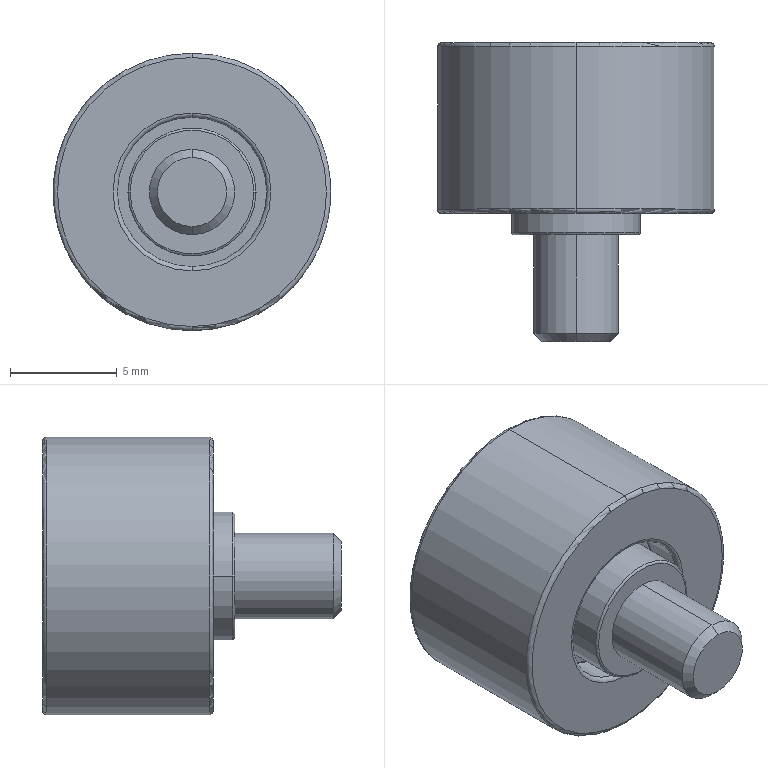Part | SolidWorks | features Fillet 4, ICE 2, Revolution 2, StudWizard 1 | 3 solids | 67 faces | box 13 x 14 x 13 mm | volume 1049 mm3 | torus 24 | cylinder 24 | plane 17 | cone 2 | commonest cylinder face diameters 0.2 x6 4 x6 7 x4 9 x4 6 x2 13 x2